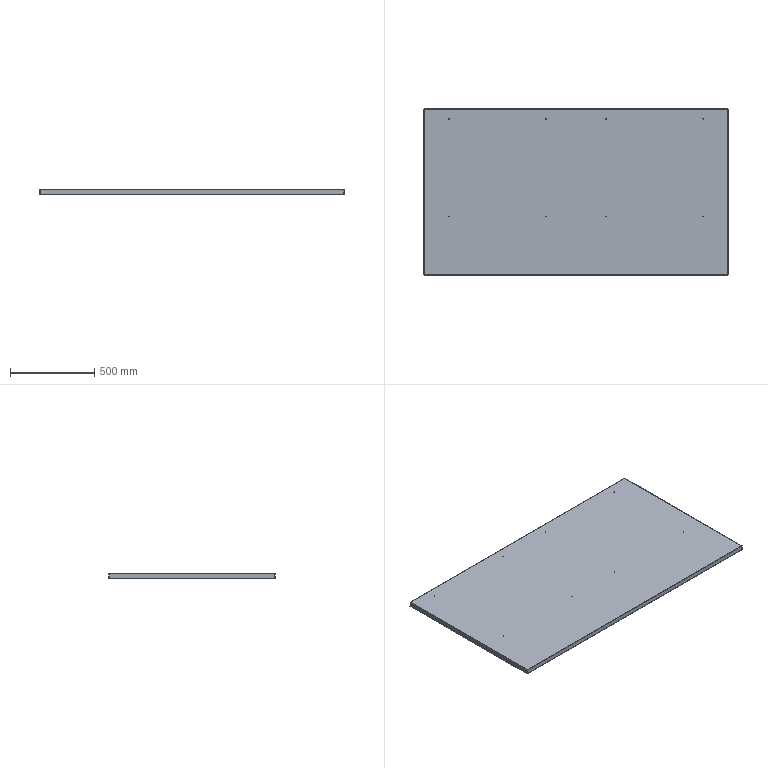Part | SolidWorks | features EdgeFlange 2, LPattern 2, FlatPattern 1, HoleWzd 1, SMBaseFlange 1, SheetMetal 1 | 1 solid | 86 faces | box 1809 x 989 x 30 mm | volume 3065759 mm3 | plane 38 | cylinder 32 | spline 16 | commonest cylinder face diameters 3.3 x16 1 x8 4 x8